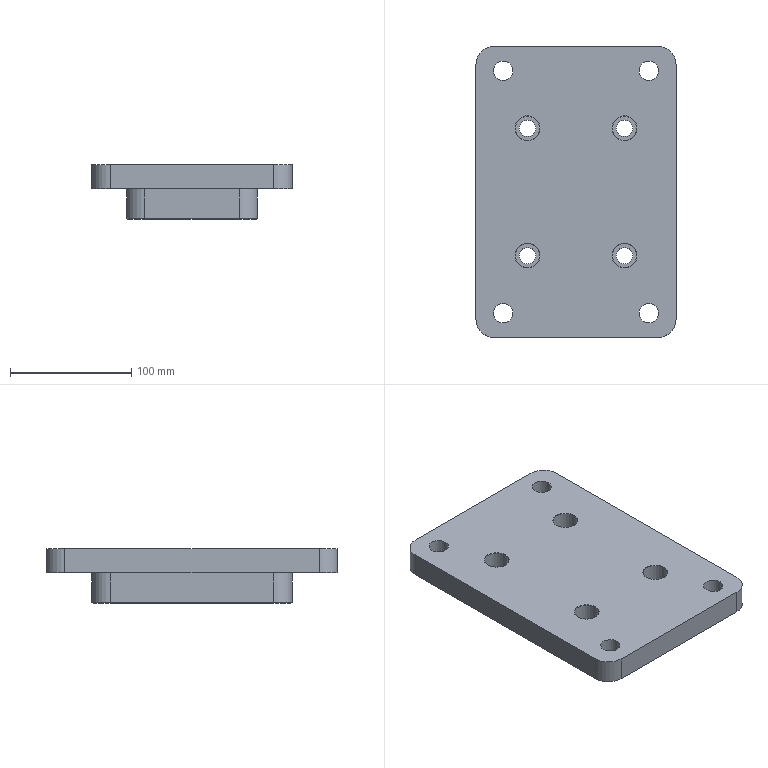NC program | NX | posted with a generic post | part box 165 x 240 x 45 mm
Lines 2078 to 2364 of 2364:
(FLOOR_WALL , TOOL : D10JING)
N4142 T11 M6
N4144 G54
N4146 G17 G0 G90 X-122.613 Y82.291 S5000 M3
N4148 G43 Z30. H11
N4150 Z-22.
N4152 G95 G1 Z-25. F3.
N4154 X-118.407 Y82.341
N4156 G94 X114.467 Y85.117 F1200.
N4158 G2 X120.423 Y80.234 R20.
N4160 G1 X-122.413 Y77.338
N4162 G3 X-124.401 Y72.36 R20.
N4164 G1 X123.41 Y75.314
N4166 G2 X124.792 Y70.376 R20.
N4168 G1 X-125. Y67.398
N4170 Y62.444
N4172 X125. Y65.424
N4174 Y60.469
N4176 X43.691 Y59.5
N4178 X67.5
N4180 G2 X80.338 Y54.982 R20.5
N4182 G1 X125. Y55.515
N4184 Y50.56
N4186 X84.748 Y50.08
N4188 G2 X87.055 Y45.153 R20.5
N4190 G1 X125. Y45.605
N4192 Y40.651
N4194 X87.964 Y40.209
N4196 G2 X88. Y39. R20.5
N4198 G1 Y35.255
N4200 X125. Y35.696
N4202 Y30.741
N4204 X88. Y30.3
N4206 Y25.345
N4208 X125. Y25.787
N4210 Y20.832
N4212 X88. Y20.391
N4214 Y15.436
N4216 X125. Y15.877
N4218 Y10.922
N4220 X88. Y10.481
N4222 Y5.527
N4224 X125. Y5.968
N4226 Y1.013
N4228 X88. Y0.572
N4230 Y-4.383
N4232 X125. Y-3.942
N4234 Y-8.896
N4236 X88. Y-9.337
N4238 Y-14.292
N4240 X125. Y-13.851
N4242 Y-18.806
N4244 X88. Y-19.247
N4246 Y-24.202
N4248 X125. Y-23.76
N4250 Y-28.715
N4252 X88. Y-29.156
N4254 Y-34.111
N4256 X125. Y-33.67
N4258 Y-38.624
N4260 X88. Y-39.066
N4262 G2 X87.374 Y-44.028 R20.5
N4264 G1 X125. Y-43.579
N4266 Y-48.534
N4268 X85.392 Y-49.006
N4270 G2 X81.465 Y-54.008 R20.5
N4272 G1 X125. Y-53.489
N4274 Y-58.443
N4276 X71.631 Y-59.08
N4278 Z-22.
N4280 G0 Z30.
N4282 X43.691 Y59.5
N4284 Z-22.
N4286 G95 G1 Z-25. F3.
N4288 X-67.5
N4290 G3 X-74.984 Y58.085 R20.5
N4292 G94 G1 X-125. Y57.489 F1200.
N4294 Y52.534
N4296 X-82.436 Y53.042
N4298 G3 X-85.896 Y48.046 R20.5
N4300 G1 X-125. Y47.579
N4302 Y42.625
N4304 X-87.592 Y43.071
N4306 G3 X-88. Y39. R20.5
N4308 G1 Y38.111
N4310 X-125. Y37.67
N4312 Y32.715
N4314 X-88. Y33.157
N4316 Y28.202
N4318 X-125. Y27.761
N4320 Y22.806
N4322 X-88. Y23.247
N4324 Y18.292
N4326 X-125. Y17.851
N4328 Y12.897
N4330 X-88. Y13.338
N4332 Y8.383
N4334 X-125. Y7.942
N4336 Y2.987
N4338 X-88. Y3.428
N4340 Y-1.526
N4342 X-125. Y-1.967
N4344 Y-6.922
N4346 X-88. Y-6.481
N4348 Y-11.436
N4350 X-125. Y-11.877
N4352 Y-16.832
N4354 X-88. Y-16.39
N4356 Y-21.345
N4358 X-125. Y-21.786
N4360 Y-26.741
N4362 X-88. Y-26.3
N4364 Y-31.255
N4366 X-125. Y-31.696
N4368 Y-36.65
N4370 X-88. Y-36.209
N4372 Y-39.
N4374 G3 X-87.886 Y-41.163 R20.5
N4376 G1 X-125. Y-41.605
N4378 Y-46.56
N4380 X-86.73 Y-46.103
N4382 G3 X-84.101 Y-51.027 R20.5
N4384 G1 X-125. Y-51.514
N4386 Y-56.469
N4388 X-79.072 Y-55.922
N4390 G3 X-67.5 Y-59.5 R20.5
N4392 G1 X36.363
N4394 X-125. Y-61.424
N4396 Y-66.378
N4398 X125. Y-63.398
N4400 Y-67.5
N4402 G2 X124.982 Y-68.353 R20.
N4404 G1 X-124.63 Y-71.329
N4406 G3 X-122.978 Y-76.264 R20.
N4408 G1 X124.135 Y-73.318
N4410 G2 X121.833 Y-78.3 R20.
N4412 G1 X-119.591 Y-81.178
N4414 X-123.457 Y-81.224
N4416 Z-22.
N4418 G0 Z30.
N4420 X0. Y-62.5
N4422 Z-22.
N4424 G95 G1 Z-25. F3.
N4426 Y-59.
N4428 G94 X-67.5 F1200.
N4430 G2 X-87.5 Y-39. R20.
N4432 G1 Y39.
N4434 G2 X-67.5 Y59. R20.
N4436 G1 X67.5
N4438 G2 X87.5 Y39. R20.
N4440 G1 Y-39.
N4442 G2 X67.5 Y-59. R20.
N4444 G1 X0.
N4446 Y-62.5
N4448 Z-22.
N4450 G0 Z30.
N4452 M5
(PLANAR_MILL_COPY_COPY_COPY , TOOL : D6A45)
N4454 T07 M6
N4456 G54
N4458 G17 G0 G90 X54.315 Y43.843 S7500 M3
N4460 G43 Z30. H7
N4462 Z1.5
N4464 G94 G1 Z-1.5 F1250.
N4466 X53.266 Y45.093
N4468 G3 X52.5 Y45.45 R1.
N4470 X47.05 Y40. R5.45
N4472 X52.5 Y45.45 R-5.45
N4474 X51.734 Y45.093 R1.
N4476 G1 X50.685 Y43.843
N4478 Z1.5
N4480 G0 Z30.
N4482 Y-43.843
N4484 Z1.5
N4486 G1 Z-1.5
N4488 X51.734 Y-45.093
N4490 G3 X52.5 Y-45.45 R1.
N4492 X57.95 Y-40. R5.45
N4494 X52.5 Y-45.45 R-5.45
N4496 X53.266 Y-45.093 R1.
N4498 G1 X54.315 Y-43.843
N4500 Z1.5
N4502 G0 Z30.
N4504 X-54.315
N4506 Z1.5
N4508 G1 Z-1.5
N4510 X-53.266 Y-45.093
N4512 G3 X-52.5 Y-45.45 R1.
N4514 X-47.05 Y-40. R5.45
N4516 X-52.5 Y-45.45 R-5.45
N4518 X-51.734 Y-45.093 R1.
N4520 G1 X-50.685 Y-43.843
N4522 Z1.5
N4524 G0 Z30.
N4526 Y43.843
N4528 Z1.5
N4530 G1 Z-1.5
N4532 X-51.734 Y45.093
N4534 G3 X-52.5 Y45.45 R1.
N4536 X-57.95 Y40. R5.45
N4538 X-52.5 Y45.45 R-5.45
N4540 X-53.266 Y45.093 R1.
N4542 G1 X-54.315 Y43.843
N4544 Z1.5
N4546 G0 Z30.
(PLANAR_MILL_COPY_COPY_COPY_COPY , TOOL : D6A45)
N4548 X-1.473 Y56.2
N4550 Z1.
N4552 G1 Z-2.
N4554 X-0.766 Y55.357
N4556 G3 X0. Y55. R1.
N4558 G1 X67.5
N4560 G2 X83.5 Y39. R16.
N4562 G1 Y-39.
N4564 G2 X67.5 Y-55. R16.
N4566 G1 X-67.5
N4568 G2 X-83.5 Y-39. R16.
N4570 G1 Y39.
N4572 G2 X-67.5 Y55. R16.
N4574 G1 X0.
N4576 G3 X0.766 Y55.357 R1.
N4578 G1 X1.473 Y56.2
N4580 Z1.
N4582 G0 Z30.
(PLANAR_MILL_COPY_COPY_COPY_COPY_1 , TOOL : D6A45)
N4584 X-99.234 Y66.343
N4586 Z-23.5
N4588 G1 Z-26.5
N4590 G3 X-100. Y66.7 R1.
N4592 X-106.7 Y60. R6.7
N4594 X-100. Y66.7 R-6.7
N4596 X-100.766 Y66.343 R1.
N4598 G1 Z-23.5
N4600 G0 Z30.
N4602 X-106.343 Y-59.234
N4604 Z-23.5
N4606 G1 Z-26.5
N4608 G3 X-106.7 Y-60. R1.
N4610 X-100. Y-66.7 R6.7
N4612 X-106.7 Y-60. R-6.7
N4614 X-106.343 Y-60.766 R1.
N4616 G1 Z-23.5
N4618 G0 Z30.
N4620 X0.766 Y-84.157
N4622 Z-23.5
N4624 G1 Z-26.5
N4626 G3 X0. Y-83.8 R1.
N4628 G1 X-105.
N4630 G2 X-121.3 Y-67.5 R16.3
N4632 G1 Y67.5
N4634 G2 X-105. Y83.8 R16.3
N4636 G1 X105.
N4638 G2 X121.3 Y67.5 R16.3
N4640 G1 Y-67.5
N4642 G2 X105. Y-83.8 R16.3
N4644 G1 X0.
N4646 G3 X-0.766 Y-84.157 R1.
N4648 G1 Z-23.5
N4650 G0 Z30.
N4652 X99.234 Y-66.343
N4654 Z-23.5
N4656 G1 Z-26.5
N4658 G3 X100. Y-66.7 R1.
N4660 X106.7 Y-60. R6.7
N4662 X100. Y-66.7 R-6.7
N4664 X100.766 Y-66.343 R1.
N4666 G1 Z-23.5
N4668 G0 Z30.
N4670 X106.343 Y59.234
N4672 Z-23.5
N4674 G1 Z-26.5
N4676 G3 X106.7 Y60. R1.
N4678 X100. Y66.7 R6.7
N4680 X106.7 Y60. R-6.7
N4682 X106.343 Y60.766 R1.
N4684 G1 Z-23.5
N4686 G0 Z30.
N4688 M5
N4690 M2